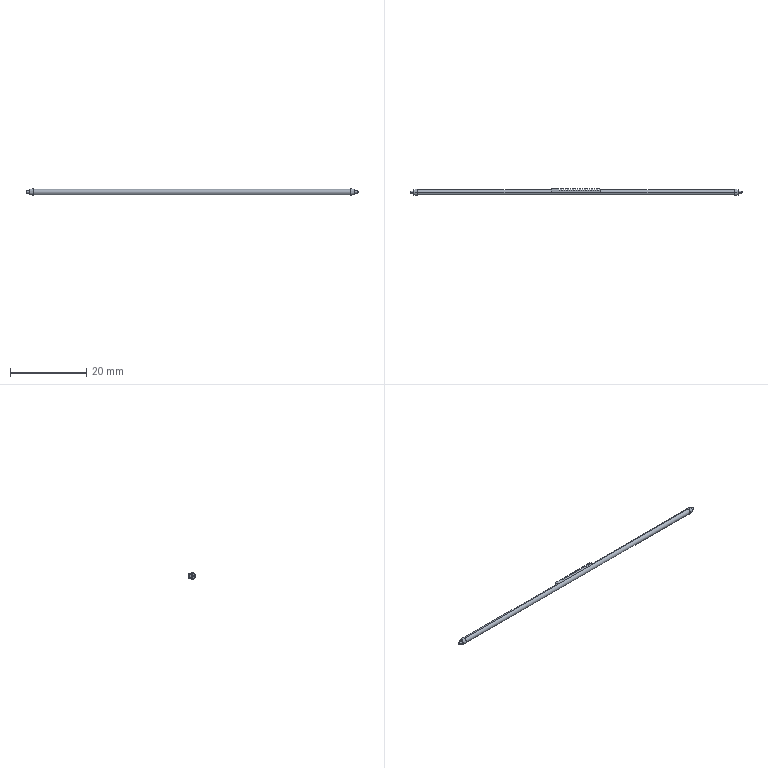Part | SolidWorks | features ICE 6, Extrusion 1, Fillet 1, LPattern 1, MirrorPattern 1 | 1 solid | 99 faces | box 87 x 1.829 x 1.659 mm | volume 137.092 mm3 | plane 84 | cylinder 7 | torus 4 | cone 4 | commonest cylinder face diameters 0.66 x4 1.4 x3